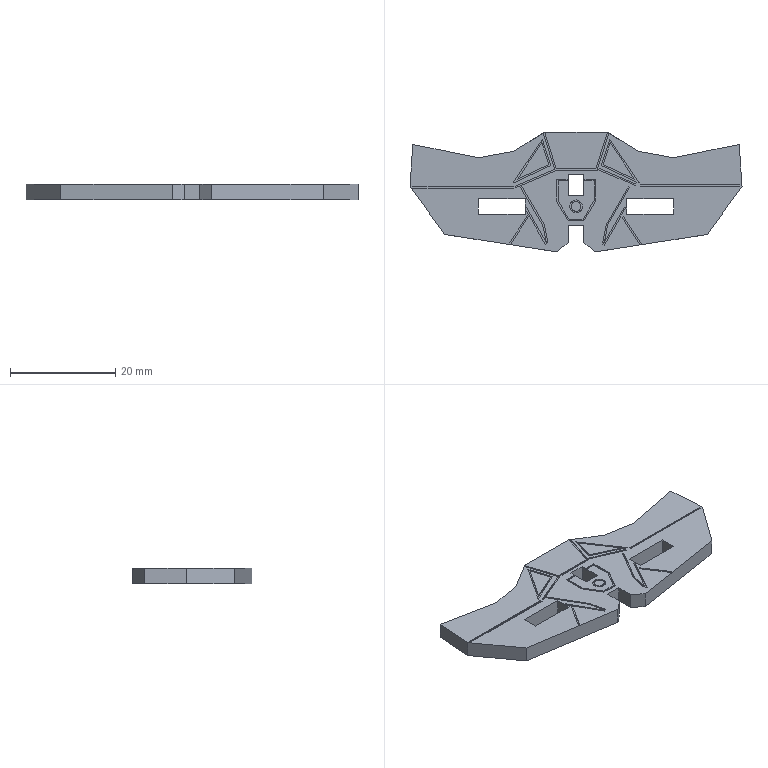Part | SolidWorks | features BaseBody 1 | 1 solid | 136 faces | box 62.988 x 22.726 x 3 mm | volume 2983 mm3 | plane 116 | spline 20